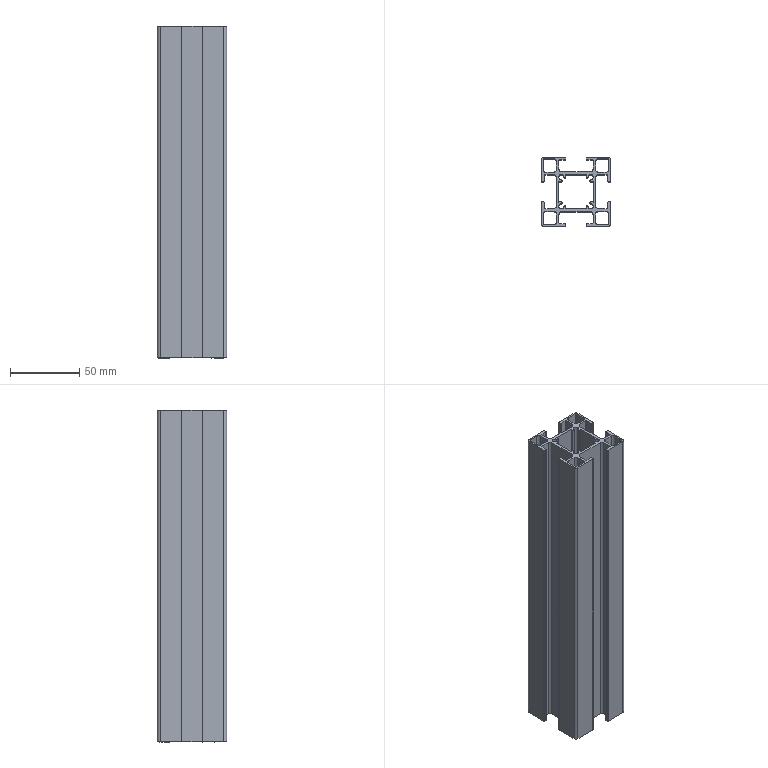Part | STEP file | 46A-00006CC11-240mm | 1 solid | 142 faces | box 50 x 50 x 240 mm | volume 140998 mm3 | cylinder 84 | plane 58 | commonest cylinder face diameters 1 x24 4 x24 1.5 x16 3.7 x8 6.7 x8 2 x4